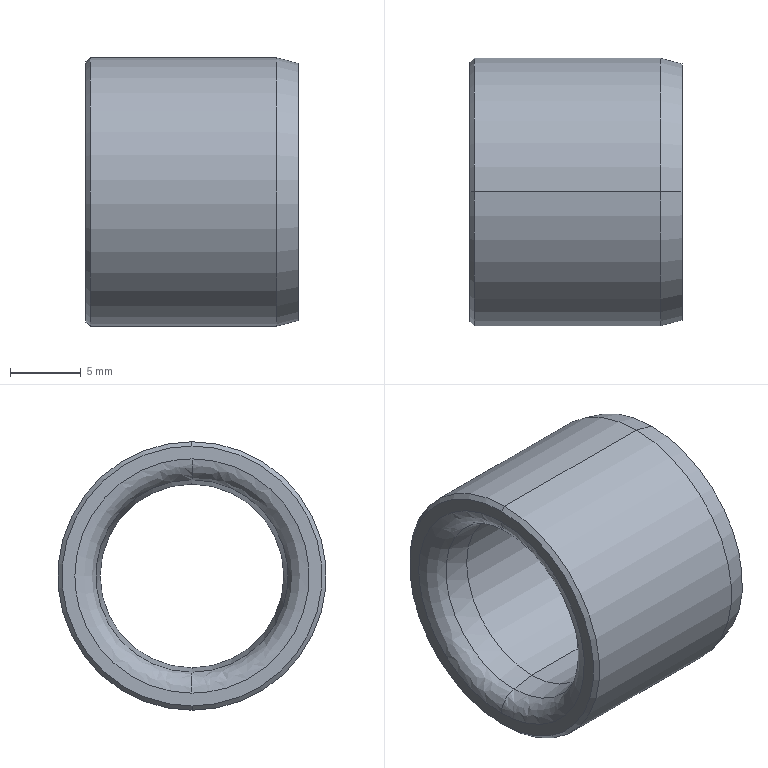Part | STEP file | TQ-DD-1105WWmpbz13_15_2_031010 | 1 solid | 18 faces | box 15 x 19 x 19 mm | volume 2146 mm3 | cone 8 | spline 4 | cylinder 4 | plane 2 | commonest cylinder face diameters 13 x2 19 x2
STEP:
#1=CARTESIAN_POINT('',(1.24,0.,6.81));
#2=VERTEX_POINT('',#1);
#3=CARTESIAN_POINT('',(1.24,0.,-6.81));
#4=VERTEX_POINT('',#3);
#5=CARTESIAN_POINT('',(1.24,0.,0.));
#6=DIRECTION('',(1.,0.,0.));
#7=DIRECTION('',(0.,0.,1.));
#8=AXIS2_PLACEMENT_3D('',#5,#6,#7);
#9=CIRCLE('',#8,6.81);
#10=EDGE_CURVE('',#2,#4,#9,.T.);
#11=ORIENTED_EDGE('',*,*,#10,.T.);
#12=CARTESIAN_POINT('',(0.,0.,-8.288));
#13=VERTEX_POINT('',#12);
#14=CARTESIAN_POINT('',(1.5,0.,-8.288));
#15=DIRECTION('',(0.,-1.,0.));
#16=DIRECTION('',(0.,0.,-1.));
#17=AXIS2_PLACEMENT_3D('',#14,#15,#16);
#18=CIRCLE('',#17,1.5);
#19=EDGE_CURVE('',#4,#13,#18,.T.);
#20=ORIENTED_EDGE('',*,*,#19,.T.);
#21=CARTESIAN_POINT('',(0.,0.,8.288));
#22=VERTEX_POINT('',#21);
#23=CARTESIAN_POINT('',(0.,0.,8.288));
#24=CARTESIAN_POINT('',(0.,-0.2535,8.288));
#25=CARTESIAN_POINT('',(0.,-0.6322,8.27));
#26=CARTESIAN_POINT('',(0.,-1.071,8.22));
#27=CARTESIAN_POINT('',(0.,-1.29,8.187));
#28=CARTESIAN_POINT('',(0.,-1.383,8.171));
#29=CARTESIAN_POINT('',(0.,-1.446,8.161));
#30=CARTESIAN_POINT('',(0.,-1.475,8.155));
#31=CARTESIAN_POINT('',(0.,-1.772,8.1));
#32=CARTESIAN_POINT('',(0.,-2.163,8.008));
#33=CARTESIAN_POINT('',(0.,-2.61,7.868));
#34=CARTESIAN_POINT('',(0.,-2.831,7.79));
#35=CARTESIAN_POINT('',(0.,-2.925,7.754));
#36=CARTESIAN_POINT('',(0.,-2.988,7.73));
#37=CARTESIAN_POINT('',(0.,-3.018,7.719));
#38=CARTESIAN_POINT('',(0.,-3.311,7.603));
#39=CARTESIAN_POINT('',(0.,-3.692,7.429));
#40=CARTESIAN_POINT('',(0.,-4.119,7.194));
#41=CARTESIAN_POINT('',(0.,-4.298,7.086));
#42=CARTESIAN_POINT('',(0.,-4.417,7.013));
#43=CARTESIAN_POINT('',(0.,-4.475,6.976));
#44=CARTESIAN_POINT('',(0.,-5.014,6.624));
#45=CARTESIAN_POINT('',(0.,-5.456,6.265));
#46=CARTESIAN_POINT('',(0.,-6.062,5.658));
#47=CARTESIAN_POINT('',(0.,-6.349,5.341));
#48=CARTESIAN_POINT('',(0.,-6.653,4.946));
#49=CARTESIAN_POINT('',(0.,-6.776,4.772));
#50=CARTESIAN_POINT('',(0.,-6.858,4.654));
#51=CARTESIAN_POINT('',(0.,-6.898,4.594));
#52=CARTESIAN_POINT('',(0.,-7.09,4.301));
#53=CARTESIAN_POINT('',(0.,-7.301,3.94));
#54=CARTESIAN_POINT('',(0.,-7.514,3.501));
#55=CARTESIAN_POINT('',(0.,-7.613,3.277));
#56=CARTESIAN_POINT('',(0.,-7.653,3.18));
#57=CARTESIAN_POINT('',(0.,-7.68,3.116));
#58=CARTESIAN_POINT('',(0.,-7.693,3.082));
#59=CARTESIAN_POINT('',(0.,-7.805,2.801));
#60=CARTESIAN_POINT('',(0.,-7.934,2.421));
#61=CARTESIAN_POINT('',(0.,-8.053,1.968));
#62=CARTESIAN_POINT('',(0.,-8.104,1.739));
#63=CARTESIAN_POINT('',(0.,-8.124,1.64));
#64=CARTESIAN_POINT('',(0.,-8.137,1.574));
#65=CARTESIAN_POINT('',(0.,-8.144,1.539));
#66=CARTESIAN_POINT('',(0.,-8.241,1.01));
#67=CARTESIAN_POINT('',(0.,-8.288,0.5066));
#68=CARTESIAN_POINT('',(0.,-8.288,-0.2533));
#69=CARTESIAN_POINT('',(0.,-8.27,-0.6317));
#70=CARTESIAN_POINT('',(0.,-8.22,-1.071));
#71=CARTESIAN_POINT('',(0.,-8.187,-1.29));
#72=CARTESIAN_POINT('',(0.,-8.171,-1.383));
#73=CARTESIAN_POINT('',(0.,-8.161,-1.446));
#74=CARTESIAN_POINT('',(0.,-8.155,-1.475));
#75=CARTESIAN_POINT('',(0.,-8.1,-1.772));
#76=CARTESIAN_POINT('',(0.,-8.008,-2.163));
#77=CARTESIAN_POINT('',(0.,-7.868,-2.61));
#78=CARTESIAN_POINT('',(0.,-7.79,-2.831));
#79=CARTESIAN_POINT('',(0.,-7.754,-2.925));
#80=CARTESIAN_POINT('',(0.,-7.73,-2.988));
#81=CARTESIAN_POINT('',(0.,-7.719,-3.018));
#82=CARTESIAN_POINT('',(0.,-7.603,-3.311));
#83=CARTESIAN_POINT('',(0.,-7.429,-3.692));
#84=CARTESIAN_POINT('',(0.,-7.194,-4.119));
#85=CARTESIAN_POINT('',(0.,-7.086,-4.298));
#86=CARTESIAN_POINT('',(0.,-7.013,-4.417));
#87=CARTESIAN_POINT('',(0.,-6.976,-4.475));
#88=CARTESIAN_POINT('',(0.,-6.624,-5.014));
#89=CARTESIAN_POINT('',(0.,-6.265,-5.456));
#90=CARTESIAN_POINT('',(0.,-5.658,-6.062));
#91=CARTESIAN_POINT('',(0.,-5.341,-6.349));
#92=CARTESIAN_POINT('',(0.,-4.946,-6.653));
#93=CARTESIAN_POINT('',(0.,-4.772,-6.776));
#94=CARTESIAN_POINT('',(0.,-4.654,-6.858));
#95=CARTESIAN_POINT('',(0.,-4.594,-6.898));
#96=CARTESIAN_POINT('',(0.,-4.301,-7.09));
#97=CARTESIAN_POINT('',(0.,-3.94,-7.301));
#98=CARTESIAN_POINT('',(0.,-3.501,-7.514));
#99=CARTESIAN_POINT('',(0.,-3.277,-7.613));
#100=CARTESIAN_POINT('',(0.,-3.18,-7.653));
#101=CARTESIAN_POINT('',(0.,-3.116,-7.68));
#102=CARTESIAN_POINT('',(0.,-3.082,-7.693));
#103=CARTESIAN_POINT('',(0.,-2.801,-7.805));
#104=CARTESIAN_POINT('',(0.,-2.421,-7.934));
#105=CARTESIAN_POINT('',(0.,-1.968,-8.053));
#106=CARTESIAN_POINT('',(0.,-1.739,-8.104));
#107=CARTESIAN_POINT('',(0.,-1.64,-8.124));
#108=CARTESIAN_POINT('',(0.,-1.574,-8.137));
#109=CARTESIAN_POINT('',(0.,-1.539,-8.144));
#110=CARTESIAN_POINT('',(0.,-1.01,-8.241));
#111=CARTESIAN_POINT('',(0.,-0.5074,-8.288));
#112=CARTESIAN_POINT('',(0.,0.,-8.288));
#113=B_SPLINE_CURVE_WITH_KNOTS('',3,(#23,#24,#25,#26,#27,#28,#29,#30,#31,#32,#33,#34,#35,#36,#37,#38,#39,#40,#41,#42,#43,#44,#45,#46,#47,#48,#49,#50,#51,#52,#53,#54,#55,#56,#57,#58,#59,#60,#61,#62,#63,#64,#65,#66,#67,#68,#69,#70,#71,#72,#73,#74,#75,#76,#77,#78,#79,#80,#81,#82,#83,#84,#85,#86,#87,#88,#89,#90,#91,#92,#93,#94,#95,#96,#97,#98,#99,#100,#101,#102,#103,#104,#105,#106,#107,#108,#109,#110,#111,#112),.UNSPECIFIED.,.F.,.F.,(4,1,1,1,2,2,1,1,1,2,2,1,1,2,2,2,1,1,2,2,1,1,1,2,2,1,1,1,2,2,2,1,1,1,2,2,1,1,1,2,2,1,1,2,2,2,1,1,2,2,1,1,1,2,2,1,1,1,2,2,4),(0.,0.03125,0.04688,0.05469,0.05859,0.0625,0.09375,0.1094,0.1172,0.1211,0.125,0.1563,0.1719,0.1797,0.1875,0.25,0.2813,0.2969,0.3047,0.3125,0.3438,0.3594,0.3672,0.3711,0.375,0.4063,0.4219,0.4297,0.4336,0.4375,0.5,0.5313,0.5469,0.5547,0.5586,0.5625,0.5938,0.6094,0.6172,0.6211,0.625,0.6563,0.6719,0.6797,0.6875,0.75,0.7813,0.7969,0.8047,0.8125,0.8437,0.8594,0.8672,0.8711,0.875,0.9063,0.9219,0.9297,0.9336,0.9375,1.),.UNSPECIFIED.);
#114=EDGE_CURVE('',#22,#13,#113,.T.);
#115=ORIENTED_EDGE('',*,*,#114,.F.);
#116=CARTESIAN_POINT('',(1.5,0.,8.288));
#117=DIRECTION('',(0.,1.,0.));
#118=DIRECTION('',(0.,0.,1.));
#119=AXIS2_PLACEMENT_3D('',#116,#117,#118);
#120=CIRCLE('',#119,1.5);
#121=EDGE_CURVE('',#2,#22,#120,.T.);
#122=ORIENTED_EDGE('',*,*,#121,.F.);
#123=EDGE_LOOP('',(#11,#20,#115,#122));
#124=FACE_OUTER_BOUND('',#123,.T.);
#125=CARTESIAN_POINT('',(1.24,0.,-6.81));
#126=CARTESIAN_POINT('',(1.24,-13.621,-6.81));
#127=CARTESIAN_POINT('',(1.24,-13.621,6.81));
#128=CARTESIAN_POINT('',(1.24,0.,6.81));
#129=CARTESIAN_POINT('',(0.4895,0.,-6.943));
#130=CARTESIAN_POINT('',(0.4895,-13.885,-6.943));
#131=CARTESIAN_POINT('',(0.4895,-13.885,6.943));
#132=CARTESIAN_POINT('',(0.4895,0.,6.943));
#133=CARTESIAN_POINT('',(0.,0.,-7.526));
#134=CARTESIAN_POINT('',(0.,-15.052,-7.526));
#135=CARTESIAN_POINT('',(0.,-15.052,7.526));
#136=CARTESIAN_POINT('',(0.,0.,7.526));
#137=CARTESIAN_POINT('',(0.,0.,-8.288));
#138=CARTESIAN_POINT('',(0.,-16.575,-8.288));
#139=CARTESIAN_POINT('',(0.,-16.575,8.288));
#140=CARTESIAN_POINT('',(0.,0.,8.288));
#141=(BOUNDED_SURFACE()B_SPLINE_SURFACE(3,3,((#125,#126,#127,#128),(#129,#130,#131,#132),(#133,#134,#135,#136),(#137,#138,#139,#140)),.UNSPECIFIED.,.F.,.F.,.F.)B_SPLINE_SURFACE_WITH_KNOTS((4,4),(4,4),(0.,1.),(0.,1.),.UNSPECIFIED.)GEOMETRIC_REPRESENTATION_ITEM()RATIONAL_B_SPLINE_SURFACE(((1.,0.3333,0.3333,1.),(0.844,0.2813,0.2813,0.844),(0.844,0.2813,0.2813,0.844),(1.,0.3333,0.3333,1.)))REPRESENTATION_ITEM('')SURFACE());
#142=ADVANCED_FACE('',(#124),#141,.T.);
#143=CARTESIAN_POINT('',(15.,0.,-8.288));
#144=VERTEX_POINT('',#143);
#145=CARTESIAN_POINT('',(15.,0.,8.288));
#146=VERTEX_POINT('',#145);
#147=CARTESIAN_POINT('',(15.,0.,-8.288));
#148=CARTESIAN_POINT('',(15.,-0.2535,-8.288));
#149=CARTESIAN_POINT('',(15.,-0.6322,-8.27));
#150=CARTESIAN_POINT('',(15.,-1.071,-8.22));
#151=CARTESIAN_POINT('',(15.,-1.29,-8.187));
#152=CARTESIAN_POINT('',(15.,-1.383,-8.171));
#153=CARTESIAN_POINT('',(15.,-1.446,-8.161));
#154=CARTESIAN_POINT('',(15.,-1.475,-8.155));
#155=CARTESIAN_POINT('',(15.,-1.772,-8.1));
#156=CARTESIAN_POINT('',(15.,-2.163,-8.008));
#157=CARTESIAN_POINT('',(15.,-2.61,-7.868));
#158=CARTESIAN_POINT('',(15.,-2.831,-7.79));
#159=CARTESIAN_POINT('',(15.,-2.925,-7.754));
#160=CARTESIAN_POINT('',(15.,-2.988,-7.73));
#161=CARTESIAN_POINT('',(15.,-3.018,-7.719));
#162=CARTESIAN_POINT('',(15.,-3.311,-7.603));
#163=CARTESIAN_POINT('',(15.,-3.692,-7.429));
#164=CARTESIAN_POINT('',(15.,-4.119,-7.194));
#165=CARTESIAN_POINT('',(15.,-4.298,-7.086));
#166=CARTESIAN_POINT('',(15.,-4.417,-7.013));
#167=CARTESIAN_POINT('',(15.,-4.475,-6.976));
#168=CARTESIAN_POINT('',(15.,-5.014,-6.624));
#169=CARTESIAN_POINT('',(15.,-5.456,-6.265));
#170=CARTESIAN_POINT('',(15.,-6.062,-5.658));
#171=CARTESIAN_POINT('',(15.,-6.349,-5.341));
#172=CARTESIAN_POINT('',(15.,-6.653,-4.946));
#173=CARTESIAN_POINT('',(15.,-6.776,-4.772));
#174=CARTESIAN_POINT('',(15.,-6.858,-4.654));
#175=CARTESIAN_POINT('',(15.,-6.898,-4.594));
#176=CARTESIAN_POINT('',(15.,-7.09,-4.301));
#177=CARTESIAN_POINT('',(15.,-7.301,-3.94));
#178=CARTESIAN_POINT('',(15.,-7.514,-3.501));
#179=CARTESIAN_POINT('',(15.,-7.613,-3.277));
#180=CARTESIAN_POINT('',(15.,-7.653,-3.18));
#181=CARTESIAN_POINT('',(15.,-7.68,-3.116));
#182=CARTESIAN_POINT('',(15.,-7.693,-3.082));
#183=CARTESIAN_POINT('',(15.,-7.805,-2.801));
#184=CARTESIAN_POINT('',(15.,-7.934,-2.421));
#185=CARTESIAN_POINT('',(15.,-8.053,-1.968));
#186=CARTESIAN_POINT('',(15.,-8.104,-1.739));
#187=CARTESIAN_POINT('',(15.,-8.124,-1.64));
#188=CARTESIAN_POINT('',(15.,-8.137,-1.574));
#189=CARTESIAN_POINT('',(15.,-8.144,-1.539));
#190=CARTESIAN_POINT('',(15.,-8.241,-1.01));
#191=CARTESIAN_POINT('',(15.,-8.288,-0.5066));
#192=CARTESIAN_POINT('',(15.,-8.288,0.2533));
#193=CARTESIAN_POINT('',(15.,-8.27,0.6317));
#194=CARTESIAN_POINT('',(15.,-8.22,1.071));
#195=CARTESIAN_POINT('',(15.,-8.187,1.29));
#196=CARTESIAN_POINT('',(15.,-8.171,1.383));
#197=CARTESIAN_POINT('',(15.,-8.161,1.446));
#198=CARTESIAN_POINT('',(15.,-8.155,1.475));
#199=CARTESIAN_POINT('',(15.,-8.1,1.772));
#200=CARTESIAN_POINT('',(15.,-8.008,2.163));
#201=CARTESIAN_POINT('',(15.,-7.868,2.61));
#202=CARTESIAN_POINT('',(15.,-7.79,2.831));
#203=CARTESIAN_POINT('',(15.,-7.754,2.925));
#204=CARTESIAN_POINT('',(15.,-7.73,2.988));
#205=CARTESIAN_POINT('',(15.,-7.719,3.018));
#206=CARTESIAN_POINT('',(15.,-7.603,3.311));
#207=CARTESIAN_POINT('',(15.,-7.429,3.692));
#208=CARTESIAN_POINT('',(15.,-7.194,4.119));
#209=CARTESIAN_POINT('',(15.,-7.086,4.298));
#210=CARTESIAN_POINT('',(15.,-7.013,4.417));
#211=CARTESIAN_POINT('',(15.,-6.976,4.475));
#212=CARTESIAN_POINT('',(15.,-6.624,5.014));
#213=CARTESIAN_POINT('',(15.,-6.265,5.456));
#214=CARTESIAN_POINT('',(15.,-5.658,6.062));
#215=CARTESIAN_POINT('',(15.,-5.341,6.349));
#216=CARTESIAN_POINT('',(15.,-4.946,6.653));
#217=CARTESIAN_POINT('',(15.,-4.772,6.776));
#218=CARTESIAN_POINT('',(15.,-4.654,6.858));
#219=CARTESIAN_POINT('',(15.,-4.594,6.898));
#220=CARTESIAN_POINT('',(15.,-4.301,7.09));
#221=CARTESIAN_POINT('',(15.,-3.94,7.301));
#222=CARTESIAN_POINT('',(15.,-3.501,7.514));
#223=CARTESIAN_POINT('',(15.,-3.277,7.613));
#224=CARTESIAN_POINT('',(15.,-3.18,7.653));
#225=CARTESIAN_POINT('',(15.,-3.116,7.68));
#226=CARTESIAN_POINT('',(15.,-3.082,7.693));
#227=CARTESIAN_POINT('',(15.,-2.801,7.805));
#228=CARTESIAN_POINT('',(15.,-2.421,7.934));
#229=CARTESIAN_POINT('',(15.,-1.968,8.053));
#230=CARTESIAN_POINT('',(15.,-1.739,8.104));
#231=CARTESIAN_POINT('',(15.,-1.64,8.124));
#232=CARTESIAN_POINT('',(15.,-1.574,8.137));
#233=CARTESIAN_POINT('',(15.,-1.539,8.144));
#234=CARTESIAN_POINT('',(15.,-1.01,8.241));
#235=CARTESIAN_POINT('',(15.,-0.5074,8.288));
#236=CARTESIAN_POINT('',(15.,0.,8.288));
#237=B_SPLINE_CURVE_WITH_KNOTS('',3,(#147,#148,#149,#150,#151,#152,#153,#154,#155,#156,#157,#158,#159,#160,#161,#162,#163,#164,#165,#166,#167,#168,#169,#170,#171,#172,#173,#174,#175,#176,#177,#178,#179,#180,#181,#182,#183,#184,#185,#186,#187,#188,#189,#190,#191,#192,#193,#194,#195,#196,#197,#198,#199,#200,#201,#202,#203,#204,#205,#206,#207,#208,#209,#210,#211,#212,#213,#214,#215,#216,#217,#218,#219,#220,#221,#222,#223,#224,#225,#226,#227,#228,#229,#230,#231,#232,#233,#234,#235,#236),.UNSPECIFIED.,.F.,.F.,(4,1,1,1,2,2,1,1,1,2,2,1,1,2,2,2,1,1,2,2,1,1,1,2,2,1,1,1,2,2,2,1,1,1,2,2,1,1,1,2,2,1,1,2,2,2,1,1,2,2,1,1,1,2,2,1,1,1,2,2,4),(0.,0.03125,0.04687,0.05469,0.05859,0.0625,0.09375,0.1094,0.1172,0.1211,0.125,0.1563,0.1719,0.1797,0.1875,0.25,0.2813,0.2969,0.3047,0.3125,0.3437,0.3594,0.3672,0.3711,0.375,0.4062,0.4219,0.4297,0.4336,0.4375,0.5,0.5312,0.5469,0.5547,0.5586,0.5625,0.5937,0.6094,0.6172,0.6211,0.625,0.6562,0.6719,0.6797,0.6875,0.75,0.7812,0.7969,0.8047,0.8125,0.8438,0.8594,0.8672,0.8711,0.875,0.9063,0.9219,0.9297,0.9336,0.9375,1.),.UNSPECIFIED.);
#238=EDGE_CURVE('',#144,#146,#237,.T.);
#239=ORIENTED_EDGE('',*,*,#238,.F.);
#240=CARTESIAN_POINT('',(13.76,0.,-6.81));
#241=VERTEX_POINT('',#240);
#242=CARTESIAN_POINT('',(13.5,0.,-8.288));
#243=DIRECTION('',(0.,-1.,0.));
#244=DIRECTION('',(0.,0.,-1.));
#245=AXIS2_PLACEMENT_3D('',#242,#243,#244);
#246=CIRCLE('',#245,1.5);
#247=EDGE_CURVE('',#144,#241,#246,.T.);
#248=ORIENTED_EDGE('',*,*,#247,.T.);
#249=CARTESIAN_POINT('',(13.76,0.,6.81));
#250=VERTEX_POINT('',#249);
#251=CARTESIAN_POINT('',(13.76,0.,0.));
#252=DIRECTION('',(-1.,0.,0.));
#253=DIRECTION('',(0.,0.,1.));
#254=AXIS2_PLACEMENT_3D('',#251,#252,#253);
#255=CIRCLE('',#254,6.81);
#256=EDGE_CURVE('',#241,#250,#255,.T.);
#257=ORIENTED_EDGE('',*,*,#256,.T.);
#258=CARTESIAN_POINT('',(13.5,0.,8.288));
#259=DIRECTION('',(0.,1.,0.));
#260=DIRECTION('',(0.,0.,1.));
#261=AXIS2_PLACEMENT_3D('',#258,#259,#260);
#262=CIRCLE('',#261,1.5);
#263=EDGE_CURVE('',#146,#250,#262,.T.);
#264=ORIENTED_EDGE('',*,*,#263,.F.);
#265=EDGE_LOOP('',(#239,#248,#257,#264));
#266=FACE_OUTER_BOUND('',#265,.T.);
#267=CARTESIAN_POINT('',(15.,0.,-8.288));
#268=CARTESIAN_POINT('',(15.,-16.575,-8.288));
#269=CARTESIAN_POINT('',(15.,-16.575,8.288));
#270=CARTESIAN_POINT('',(15.,0.,8.288));
#271=CARTESIAN_POINT('',(15.,0.,-7.526));
#272=CARTESIAN_POINT('',(15.,-15.052,-7.526));
#273=CARTESIAN_POINT('',(15.,-15.052,7.526));
#274=CARTESIAN_POINT('',(15.,0.,7.526));
#275=CARTESIAN_POINT('',(14.51,0.,-6.943));
#276=CARTESIAN_POINT('',(14.51,-13.885,-6.943));
#277=CARTESIAN_POINT('',(14.51,-13.885,6.943));
#278=CARTESIAN_POINT('',(14.51,0.,6.943));
#279=CARTESIAN_POINT('',(13.76,0.,-6.81));
#280=CARTESIAN_POINT('',(13.76,-13.621,-6.81));
#281=CARTESIAN_POINT('',(13.76,-13.621,6.81));
#282=CARTESIAN_POINT('',(13.76,0.,6.81));
#283=(BOUNDED_SURFACE()B_SPLINE_SURFACE(3,3,((#267,#268,#269,#270),(#271,#272,#273,#274),(#275,#276,#277,#278),(#279,#280,#281,#282)),.UNSPECIFIED.,.F.,.F.,.F.)B_SPLINE_SURFACE_WITH_KNOTS((4,4),(4,4),(0.,1.),(0.,1.),.UNSPECIFIED.)GEOMETRIC_REPRESENTATION_ITEM()RATIONAL_B_SPLINE_SURFACE(((1.,0.3333,0.3333,1.),(0.844,0.2813,0.2813,0.844),(0.844,0.2813,0.2813,0.844),(1.,0.3333,0.3333,1.)))REPRESENTATION_ITEM('')SURFACE());
#284=ADVANCED_FACE('',(#266),#283,.T.);
#285=CARTESIAN_POINT('',(0.3,0.,-9.5));
#286=VERTEX_POINT('',#285);
#287=CARTESIAN_POINT('',(0.3,0.,9.5));
#288=VERTEX_POINT('',#287);
#289=CARTESIAN_POINT('',(0.3,0.,0.));
#290=DIRECTION('',(1.,0.,0.));
#291=DIRECTION('',(0.,0.,-1.));
#292=AXIS2_PLACEMENT_3D('',#289,#290,#291);
#293=CIRCLE('',#292,9.5);
#294=EDGE_CURVE('',#286,#288,#293,.T.);
#295=ORIENTED_EDGE('',*,*,#294,.T.);
#296=CARTESIAN_POINT('',(13.5,0.,9.5));
#297=VERTEX_POINT('',#296);
#298=CARTESIAN_POINT('',(6.9,0.,9.5));
#299=DIRECTION('',(1.,0.,0.));
#300=VECTOR('',#299,1000.);
#301=LINE('',#298,#300);
#302=EDGE_CURVE('',#288,#297,#301,.T.);
#303=ORIENTED_EDGE('',*,*,#302,.T.);
#304=CARTESIAN_POINT('',(13.5,0.,-9.5));
#305=VERTEX_POINT('',#304);
#306=CARTESIAN_POINT('',(13.5,0.,0.));
#307=DIRECTION('',(-1.,0.,0.));
#308=DIRECTION('',(0.,0.,-1.));
#309=AXIS2_PLACEMENT_3D('',#306,#307,#308);
#310=CIRCLE('',#309,9.5);
#311=EDGE_CURVE('',#297,#305,#310,.T.);
#312=ORIENTED_EDGE('',*,*,#311,.T.);
#313=CARTESIAN_POINT('',(6.9,0.,-9.5));
#314=DIRECTION('',(1.,0.,0.));
#315=VECTOR('',#314,1000.);
#316=LINE('',#313,#315);
#317=EDGE_CURVE('',#286,#305,#316,.T.);
#318=ORIENTED_EDGE('',*,*,#317,.F.);
#319=EDGE_LOOP('',(#295,#303,#312,#318));
#320=FACE_OUTER_BOUND('',#319,.T.);
#321=CARTESIAN_POINT('',(6.9,0.,0.));
#322=DIRECTION('',(1.,0.,0.));
#323=DIRECTION('',(0.,0.,-1.));
#324=AXIS2_PLACEMENT_3D('',#321,#322,#323);
#325=CYLINDRICAL_SURFACE('',#324,9.5);
#326=ADVANCED_FACE('',(#320),#325,.T.);
#327=CARTESIAN_POINT('',(0.,0.,-9.2));
#328=VERTEX_POINT('',#327);
#329=CARTESIAN_POINT('',(0.,0.,9.2));
#330=VERTEX_POINT('',#329);
#331=CARTESIAN_POINT('',(0.,0.,0.));
#332=DIRECTION('',(1.,0.,0.));
#333=DIRECTION('',(0.,0.,-1.));
#334=AXIS2_PLACEMENT_3D('',#331,#332,#333);
#335=CIRCLE('',#334,9.2);
#336=EDGE_CURVE('',#328,#330,#335,.T.);
#337=ORIENTED_EDGE('',*,*,#336,.T.);
#338=CARTESIAN_POINT('',(0.3,0.,9.5));
#339=DIRECTION('',(0.7071,0.,0.7071));
#340=VECTOR('',#339,1000.);
#341=LINE('',#338,#340);
#342=EDGE_CURVE('',#330,#288,#341,.T.);
#343=ORIENTED_EDGE('',*,*,#342,.T.);
#344=ORIENTED_EDGE('',*,*,#294,.F.);
#345=CARTESIAN_POINT('',(0.3,0.,-9.5));
#346=DIRECTION('',(0.7071,0.,-0.7071));
#347=VECTOR('',#346,1000.);
#348=LINE('',#345,#347);
#349=EDGE_CURVE('',#328,#286,#348,.T.);
#350=ORIENTED_EDGE('',*,*,#349,.F.);
#351=EDGE_LOOP('',(#337,#343,#344,#350));
#352=FACE_OUTER_BOUND('',#351,.T.);
#353=CARTESIAN_POINT('',(0.3,0.,0.));
#354=DIRECTION('',(1.,0.,0.));
#355=DIRECTION('',(0.,0.,-1.));
#356=AXIS2_PLACEMENT_3D('',#353,#354,#355);
#357=CONICAL_SURFACE('',#356,9.5,0.7854);
#358=ADVANCED_FACE('',(#352),#357,.T.);
#359=CARTESIAN_POINT('',(15.,0.,9.098));
#360=VERTEX_POINT('',#359);
#361=CARTESIAN_POINT('',(15.,0.,-9.098));
#362=VERTEX_POINT('',#361);
#363=CARTESIAN_POINT('',(15.,0.,0.));
#364=DIRECTION('',(-1.,0.,0.));
#365=DIRECTION('',(0.,0.,1.));
#366=AXIS2_PLACEMENT_3D('',#363,#364,#365);
#367=CIRCLE('',#366,9.098);
#368=EDGE_CURVE('',#360,#362,#367,.T.);
#369=ORIENTED_EDGE('',*,*,#368,.T.);
#370=CARTESIAN_POINT('',(13.5,0.,-9.5));
#371=DIRECTION('',(-0.9659,0.,-0.2588));
#372=VECTOR('',#371,1000.);
#373=LINE('',#370,#372);
#374=EDGE_CURVE('',#362,#305,#373,.T.);
#375=ORIENTED_EDGE('',*,*,#374,.T.);
#376=ORIENTED_EDGE('',*,*,#311,.F.);
#377=CARTESIAN_POINT('',(13.5,0.,9.5));
#378=DIRECTION('',(-0.9659,0.,0.2588));
#379=VECTOR('',#378,1000.);
#380=LINE('',#377,#379);
#381=EDGE_CURVE('',#360,#297,#380,.T.);
#382=ORIENTED_EDGE('',*,*,#381,.F.);
#383=EDGE_LOOP('',(#369,#375,#376,#382));
#384=FACE_OUTER_BOUND('',#383,.T.);
#385=CARTESIAN_POINT('',(13.5,0.,0.));
#386=DIRECTION('',(-1.,0.,0.));
#387=DIRECTION('',(0.,0.,1.));
#388=AXIS2_PLACEMENT_3D('',#385,#386,#387);
#389=CONICAL_SURFACE('',#388,9.5,0.2618);
#390=ADVANCED_FACE('',(#384),#389,.T.);
#391=CARTESIAN_POINT('',(3.,0.,-6.5));
#392=VERTEX_POINT('',#391);
#393=CARTESIAN_POINT('',(3.,0.,6.5));
#394=VERTEX_POINT('',#393);
#395=CARTESIAN_POINT('',(3.,0.,0.));
#396=DIRECTION('',(-1.,0.,0.));
#397=DIRECTION('',(0.,1.,0.));
#398=AXIS2_PLACEMENT_3D('',#395,#396,#397);
#399=CIRCLE('',#398,6.5);
#400=EDGE_CURVE('',#392,#394,#399,.T.);
#401=ORIENTED_EDGE('',*,*,#400,.F.);
#402=CARTESIAN_POINT('',(1.24,0.,-6.81));
#403=DIRECTION('',(-0.9848,0.,-0.1736));
#404=VECTOR('',#403,1000.);
#405=LINE('',#402,#404);
#406=EDGE_CURVE('',#392,#4,#405,.T.);
#407=ORIENTED_EDGE('',*,*,#406,.T.);
#408=ORIENTED_EDGE('',*,*,#10,.F.);
#409=CARTESIAN_POINT('',(1.24,0.,6.81));
#410=DIRECTION('',(-0.9848,0.,0.1736));
#411=VECTOR('',#410,1000.);
#412=LINE('',#409,#411);
#413=EDGE_CURVE('',#394,#2,#412,.T.);
#414=ORIENTED_EDGE('',*,*,#413,.F.);
#415=EDGE_LOOP('',(#401,#407,#408,#414));
#416=FACE_OUTER_BOUND('',#415,.T.);
#417=CARTESIAN_POINT('',(1.24,0.,0.));
#418=DIRECTION('',(-1.,0.,0.));
#419=DIRECTION('',(0.,0.,1.));
#420=AXIS2_PLACEMENT_3D('',#417,#418,#419);
#421=CONICAL_SURFACE('',#420,6.81,0.1745);
#422=ADVANCED_FACE('',(#416),#421,.F.);
#423=CARTESIAN_POINT('',(12.,0.,6.5));
#424=VERTEX_POINT('',#423);
#425=CARTESIAN_POINT('',(12.,0.,-6.5));
#426=VERTEX_POINT('',#425);
#427=CARTESIAN_POINT('',(12.,0.,0.));
#428=DIRECTION('',(1.,0.,0.));
#429=DIRECTION('',(0.,1.,0.));
#430=AXIS2_PLACEMENT_3D('',#427,#428,#429);
#431=CIRCLE('',#430,6.5);
#432=EDGE_CURVE('',#424,#426,#431,.T.);
#433=ORIENTED_EDGE('',*,*,#432,.F.);
#434=CARTESIAN_POINT('',(13.76,0.,6.81));
#435=DIRECTION('',(0.9848,0.,0.1736));
#436=VECTOR('',#435,1000.);
#437=LINE('',#434,#436);
#438=EDGE_CURVE('',#424,#250,#437,.T.);
#439=ORIENTED_EDGE('',*,*,#438,.T.);
#440=ORIENTED_EDGE('',*,*,#256,.F.);
#441=CARTESIAN_POINT('',(13.76,0.,-6.81));
#442=DIRECTION('',(0.9848,0.,-0.1736));
#443=VECTOR('',#442,1000.);
#444=LINE('',#441,#443);
#445=EDGE_CURVE('',#426,#241,#444,.T.);
#446=ORIENTED_EDGE('',*,*,#445,.F.);
#447=EDGE_LOOP('',(#433,#439,#440,#446));
#448=FACE_OUTER_BOUND('',#447,.T.);
#449=CARTESIAN_POINT('',(13.76,0.,0.));
#450=DIRECTION('',(1.,0.,0.));
#451=DIRECTION('',(0.,0.,-1.));
#452=AXIS2_PLACEMENT_3D('',#449,#450,#451);
#453=CONICAL_SURFACE('',#452,6.81,0.1745);
#454=ADVANCED_FACE('',(#448),#453,.F.);
#455=ORIENTED_EDGE('',*,*,#400,.T.);
#456=CARTESIAN_POINT('',(7.5,0.,6.5));
#457=DIRECTION('',(1.,0.,0.));
#458=VECTOR('',#457,1000.);
#459=LINE('',#456,#458);
#460=EDGE_CURVE('',#394,#424,#459,.T.);
#461=ORIENTED_EDGE('',*,*,#460,.T.);
#462=ORIENTED_EDGE('',*,*,#432,.T.);
#463=CARTESIAN_POINT('',(7.5,0.,-6.5));
#464=DIRECTION('',(1.,0.,0.));
#465=VECTOR('',#464,1000.);
#466=LINE('',#463,#465);
#467=EDGE_CURVE('',#392,#426,#466,.T.);
#468=ORIENTED_EDGE('',*,*,#467,.F.);
#469=EDGE_LOOP('',(#455,#461,#462,#468));
#470=FACE_OUTER_BOUND('',#469,.T.);
#471=CARTESIAN_POINT('',(7.5,0.,0.));
#472=DIRECTION('',(1.,0.,0.));
#473=DIRECTION('',(0.,0.,-1.));
#474=AXIS2_PLACEMENT_3D('',#471,#472,#473);
#475=CYLINDRICAL_SURFACE('',#474,6.5);
#476=ADVANCED_FACE('',(#470),#475,.F.);
#477=ORIENTED_EDGE('',*,*,#302,.F.);
#478=CARTESIAN_POINT('',(0.3,0.,0.));
#479=DIRECTION('',(1.,0.,0.));
#480=DIRECTION('',(0.,0.,-1.));
#481=AXIS2_PLACEMENT_3D('',#478,#479,#480);
#482=CIRCLE('',#481,9.5);
#483=EDGE_CURVE('',#288,#286,#482,.T.);
#484=ORIENTED_EDGE('',*,*,#483,.T.);
#485=ORIENTED_EDGE('',*,*,#317,.T.);
#486=CARTESIAN_POINT('',(13.5,0.,0.));
#487=DIRECTION('',(-1.,0.,0.));
#488=DIRECTION('',(0.,0.,-1.));
#489=AXIS2_PLACEMENT_3D('',#486,#487,#488);
#490=CIRCLE('',#489,9.5);
#491=EDGE_CURVE('',#305,#297,#490,.T.);
#492=ORIENTED_EDGE('',*,*,#491,.T.);
#493=EDGE_LOOP('',(#477,#484,#485,#492));
#494=FACE_OUTER_BOUND('',#493,.T.);
#495=CARTESIAN_POINT('',(6.9,0.,0.));
#496=DIRECTION('',(1.,0.,0.));
#497=DIRECTION('',(0.,0.,-1.));
#498=AXIS2_PLACEMENT_3D('',#495,#496,#497);
#499=CYLINDRICAL_SURFACE('',#498,9.5);
#500=ADVANCED_FACE('',(#494),#499,.T.);
#501=ORIENTED_EDGE('',*,*,#342,.F.);
#502=CARTESIAN_POINT('',(0.,0.,0.));
#503=DIRECTION('',(1.,0.,0.));
#504=DIRECTION('',(0.,0.,-1.));
#505=AXIS2_PLACEMENT_3D('',#502,#503,#504);
#506=CIRCLE('',#505,9.2);
#507=EDGE_CURVE('',#330,#328,#506,.T.);
#508=ORIENTED_EDGE('',*,*,#507,.T.);
#509=ORIENTED_EDGE('',*,*,#349,.T.);
#510=ORIENTED_EDGE('',*,*,#483,.F.);
#511=EDGE_LOOP('',(#501,#508,#509,#510));
#512=FACE_OUTER_BOUND('',#511,.T.);
#513=CARTESIAN_POINT('',(0.3,0.,0.));
#514=DIRECTION('',(1.,0.,0.));
#515=DIRECTION('',(0.,0.,-1.));
#516=AXIS2_PLACEMENT_3D('',#513,#514,#515);
#517=CONICAL_SURFACE('',#516,9.5,0.7854);
#518=ADVANCED_FACE('',(#512),#517,.T.);
#519=ORIENTED_EDGE('',*,*,#374,.F.);
#520=CARTESIAN_POINT('',(15.,0.,0.));
#521=DIRECTION('',(-1.,0.,0.));
#522=DIRECTION('',(0.,0.,1.));
#523=AXIS2_PLACEMENT_3D('',#520,#521,#522);
#524=CIRCLE('',#523,9.098);
#525=EDGE_CURVE('',#362,#360,#524,.T.);
#526=ORIENTED_EDGE('',*,*,#525,.T.);
#527=ORIENTED_EDGE('',*,*,#381,.T.);
#528=ORIENTED_EDGE('',*,*,#491,.F.);
#529=EDGE_LOOP('',(#519,#526,#527,#528));
#530=FACE_OUTER_BOUND('',#529,.T.);
#531=CARTESIAN_POINT('',(13.5,0.,0.));
#532=DIRECTION('',(-1.,0.,0.));
#533=DIRECTION('',(0.,0.,1.));
#534=AXIS2_PLACEMENT_3D('',#531,#532,#533);
#535=CONICAL_SURFACE('',#534,9.5,0.2618);
#536=ADVANCED_FACE('',(#530),#535,.T.);
#537=ORIENTED_EDGE('',*,*,#336,.F.);
#538=ORIENTED_EDGE('',*,*,#507,.F.);
#539=EDGE_LOOP('',(#537,#538));
#540=FACE_OUTER_BOUND('',#539,.T.);
#541=CARTESIAN_POINT('',(0.,8.288,0.));
#542=VERTEX_POINT('',#541);
#543=CARTESIAN_POINT('',(0.,8.288,0.));
#544=CARTESIAN_POINT('',(0.,8.288,0.2535));
#545=CARTESIAN_POINT('',(0.,8.27,0.6322));
#546=CARTESIAN_POINT('',(0.,8.22,1.071));
#547=CARTESIAN_POINT('',(0.,8.187,1.29));
#548=CARTESIAN_POINT('',(0.,8.171,1.383));
#549=CARTESIAN_POINT('',(0.,8.161,1.446));
#550=CARTESIAN_POINT('',(0.,8.155,1.475));
#551=CARTESIAN_POINT('',(0.,8.1,1.772));
#552=CARTESIAN_POINT('',(0.,8.008,2.163));
#553=CARTESIAN_POINT('',(0.,7.868,2.61));
#554=CARTESIAN_POINT('',(0.,7.79,2.831));
#555=CARTESIAN_POINT('',(0.,7.754,2.925));
#556=CARTESIAN_POINT('',(0.,7.73,2.988));
#557=CARTESIAN_POINT('',(0.,7.719,3.018));
#558=CARTESIAN_POINT('',(0.,7.603,3.311));
#559=CARTESIAN_POINT('',(0.,7.429,3.692));
#560=CARTESIAN_POINT('',(0.,7.194,4.119));
#561=CARTESIAN_POINT('',(0.,7.086,4.298));
#562=CARTESIAN_POINT('',(0.,7.013,4.417));
#563=CARTESIAN_POINT('',(0.,6.976,4.475));
#564=CARTESIAN_POINT('',(0.,6.624,5.014));
#565=CARTESIAN_POINT('',(0.,6.265,5.456));
#566=CARTESIAN_POINT('',(0.,5.658,6.062));
#567=CARTESIAN_POINT('',(0.,5.341,6.349));
#568=CARTESIAN_POINT('',(0.,4.946,6.653));
#569=CARTESIAN_POINT('',(0.,4.772,6.776));
#570=CARTESIAN_POINT('',(0.,4.654,6.858));
#571=CARTESIAN_POINT('',(0.,4.594,6.898));
#572=CARTESIAN_POINT('',(0.,4.301,7.09));
#573=CARTESIAN_POINT('',(0.,3.94,7.301));
#574=CARTESIAN_POINT('',(0.,3.501,7.514));
#575=CARTESIAN_POINT('',(0.,3.277,7.613));
#576=CARTESIAN_POINT('',(0.,3.18,7.653));
#577=CARTESIAN_POINT('',(0.,3.116,7.68));
#578=CARTESIAN_POINT('',(0.,3.082,7.693));
#579=CARTESIAN_POINT('',(0.,2.801,7.805));
#580=CARTESIAN_POINT('',(0.,2.421,7.934));
#581=CARTESIAN_POINT('',(0.,1.968,8.053));
#582=CARTESIAN_POINT('',(0.,1.739,8.104));
#583=CARTESIAN_POINT('',(0.,1.64,8.124));
#584=CARTESIAN_POINT('',(0.,1.574,8.137));
#585=CARTESIAN_POINT('',(0.,1.539,8.144));
#586=CARTESIAN_POINT('',(0.,1.01,8.241));
#587=CARTESIAN_POINT('',(0.,0.5074,8.288));
#588=CARTESIAN_POINT('',(0.,0.,8.288));
#589=B_SPLINE_CURVE_WITH_KNOTS('',3,(#543,#544,#545,#546,#547,#548,#549,#550,#551,#552,#553,#554,#555,#556,#557,#558,#559,#560,#561,#562,#563,#564,#565,#566,#567,#568,#569,#570,#571,#572,#573,#574,#575,#576,#577,#578,#579,#580,#581,#582,#583,#584,#585,#586,#587,#588),.UNSPECIFIED.,.F.,.F.,(4,1,1,1,2,2,1,1,1,2,2,1,1,2,2,2,1,1,2,2,1,1,1,2,2,1,1,1,2,2,4),(0.,0.0625,0.09375,0.1094,0.1172,0.125,0.1875,0.2188,0.2344,0.2422,0.25,0.3125,0.3438,0.3594,0.375,0.5,0.5625,0.5938,0.6094,0.625,0.6875,0.7188,0.7344,0.7422,0.75,0.8125,0.8437,0.8594,0.8672,0.875,1.),.UNSPECIFIED.);
#590=EDGE_CURVE('',#542,#22,#589,.T.);
#591=ORIENTED_EDGE('',*,*,#590,.T.);
#592=ORIENTED_EDGE('',*,*,#114,.T.);
#593=CARTESIAN_POINT('',(0.,0.,-8.288));
#594=CARTESIAN_POINT('',(0.,0.2535,-8.288));
#595=CARTESIAN_POINT('',(0.,0.6322,-8.27));
#596=CARTESIAN_POINT('',(0.,1.071,-8.22));
#597=CARTESIAN_POINT('',(0.,1.29,-8.187));
#598=CARTESIAN_POINT('',(0.,1.383,-8.171));
#599=CARTESIAN_POINT('',(0.,1.446,-8.161));
#600=CARTESIAN_POINT('',(0.,1.475,-8.155));
#601=CARTESIAN_POINT('',(0.,1.772,-8.1));
#602=CARTESIAN_POINT('',(0.,2.163,-8.008));
#603=CARTESIAN_POINT('',(0.,2.61,-7.868));
#604=CARTESIAN_POINT('',(0.,2.831,-7.79));
#605=CARTESIAN_POINT('',(0.,2.925,-7.754));
#606=CARTESIAN_POINT('',(0.,2.988,-7.73));
#607=CARTESIAN_POINT('',(0.,3.018,-7.719));
#608=CARTESIAN_POINT('',(0.,3.311,-7.603));
#609=CARTESIAN_POINT('',(0.,3.692,-7.429));
#610=CARTESIAN_POINT('',(0.,4.119,-7.194));
#611=CARTESIAN_POINT('',(0.,4.298,-7.086));
#612=CARTESIAN_POINT('',(0.,4.417,-7.013));
#613=CARTESIAN_POINT('',(0.,4.475,-6.976));
#614=CARTESIAN_POINT('',(0.,5.014,-6.624));
#615=CARTESIAN_POINT('',(0.,5.456,-6.265));
#616=CARTESIAN_POINT('',(0.,6.062,-5.658));
#617=CARTESIAN_POINT('',(0.,6.349,-5.341));
#618=CARTESIAN_POINT('',(0.,6.653,-4.946));
#619=CARTESIAN_POINT('',(0.,6.776,-4.772));
#620=CARTESIAN_POINT('',(0.,6.858,-4.654));
#621=CARTESIAN_POINT('',(0.,6.898,-4.594));
#622=CARTESIAN_POINT('',(0.,7.09,-4.301));
#623=CARTESIAN_POINT('',(0.,7.301,-3.94));
#624=CARTESIAN_POINT('',(0.,7.514,-3.501));
#625=CARTESIAN_POINT('',(0.,7.613,-3.277));
#626=CARTESIAN_POINT('',(0.,7.653,-3.18));
#627=CARTESIAN_POINT('',(0.,7.68,-3.116));
#628=CARTESIAN_POINT('',(0.,7.693,-3.082));
#629=CARTESIAN_POINT('',(0.,7.805,-2.801));
#630=CARTESIAN_POINT('',(0.,7.934,-2.421));
#631=CARTESIAN_POINT('',(0.,8.053,-1.968));
#632=CARTESIAN_POINT('',(0.,8.104,-1.739));
#633=CARTESIAN_POINT('',(0.,8.124,-1.64));
#634=CARTESIAN_POINT('',(0.,8.137,-1.574));
#635=CARTESIAN_POINT('',(0.,8.144,-1.539));
#636=CARTESIAN_POINT('',(0.,8.241,-1.01));
#637=CARTESIAN_POINT('',(0.,8.288,-0.5074));
#638=CARTESIAN_POINT('',(0.,8.288,0.));
#639=B_SPLINE_CURVE_WITH_KNOTS('',3,(#593,#594,#595,#596,#597,#598,#599,#600,#601,#602,#603,#604,#605,#606,#607,#608,#609,#610,#611,#612,#613,#614,#615,#616,#617,#618,#619,#620,#621,#622,#623,#624,#625,#626,#627,#628,#629,#630,#631,#632,#633,#634,#635,#636,#637,#638),.UNSPECIFIED.,.F.,.F.,(4,1,1,1,2,2,1,1,1,2,2,1,1,2,2,2,1,1,2,2,1,1,1,2,2,1,1,1,2,2,4),(0.,0.0625,0.09375,0.1094,0.1172,0.125,0.1875,0.2187,0.2344,0.2422,0.25,0.3125,0.3437,0.3594,0.375,0.5,0.5625,0.5937,0.6094,0.625,0.6875,0.7188,0.7344,0.7422,0.75,0.8125,0.8438,0.8594,0.8672,0.875,1.),.UNSPECIFIED.);
#640=EDGE_CURVE('',#13,#542,#639,.T.);
#641=ORIENTED_EDGE('',*,*,#640,.T.);
#642=EDGE_LOOP('',(#591,#592,#641));
#643=FACE_BOUND('',#642,.T.);
#644=CARTESIAN_POINT('',(0.,8.744,0.));
#645=DIRECTION('',(-1.,0.,0.));
#646=DIRECTION('',(0.,0.,1.));
#647=AXIS2_PLACEMENT_3D('',#644,#645,#646);
#648=PLANE('',#647);
#649=ADVANCED_FACE('',(#540,#643),#648,.T.);
#650=ORIENTED_EDGE('',*,*,#238,.T.);
#651=CARTESIAN_POINT('',(15.,8.288,0.));
#652=VERTEX_POINT('',#651);
#653=CARTESIAN_POINT('',(15.,0.,8.288));
#654=CARTESIAN_POINT('',(15.,0.2535,8.288));
#655=CARTESIAN_POINT('',(15.,0.6322,8.27));
#656=CARTESIAN_POINT('',(15.,1.071,8.22));
#657=CARTESIAN_POINT('',(15.,1.29,8.187));
#658=CARTESIAN_POINT('',(15.,1.383,8.171));
#659=CARTESIAN_POINT('',(15.,1.446,8.161));
#660=CARTESIAN_POINT('',(15.,1.475,8.155));
#661=CARTESIAN_POINT('',(15.,1.772,8.1));
#662=CARTESIAN_POINT('',(15.,2.163,8.008));
#663=CARTESIAN_POINT('',(15.,2.61,7.868));
#664=CARTESIAN_POINT('',(15.,2.831,7.79));
#665=CARTESIAN_POINT('',(15.,2.925,7.754));
#666=CARTESIAN_POINT('',(15.,2.988,7.73));
#667=CARTESIAN_POINT('',(15.,3.018,7.719));
#668=CARTESIAN_POINT('',(15.,3.311,7.603));
#669=CARTESIAN_POINT('',(15.,3.692,7.429));
#670=CARTESIAN_POINT('',(15.,4.119,7.194));
#671=CARTESIAN_POINT('',(15.,4.298,7.086));
#672=CARTESIAN_POINT('',(15.,4.417,7.013));
#673=CARTESIAN_POINT('',(15.,4.475,6.976));
#674=CARTESIAN_POINT('',(15.,5.014,6.624));
#675=CARTESIAN_POINT('',(15.,5.456,6.265));
#676=CARTESIAN_POINT('',(15.,6.062,5.658));
#677=CARTESIAN_POINT('',(15.,6.349,5.341));
#678=CARTESIAN_POINT('',(15.,6.653,4.946));
#679=CARTESIAN_POINT('',(15.,6.776,4.772));
#680=CARTESIAN_POINT('',(15.,6.858,4.654));
#681=CARTESIAN_POINT('',(15.,6.898,4.594));
#682=CARTESIAN_POINT('',(15.,7.09,4.301));
#683=CARTESIAN_POINT('',(15.,7.301,3.94));
#684=CARTESIAN_POINT('',(15.,7.514,3.501));
#685=CARTESIAN_POINT('',(15.,7.613,3.277));
#686=CARTESIAN_POINT('',(15.,7.653,3.18));
#687=CARTESIAN_POINT('',(15.,7.68,3.116));
#688=CARTESIAN_POINT('',(15.,7.693,3.082));
#689=CARTESIAN_POINT('',(15.,7.805,2.801));
#690=CARTESIAN_POINT('',(15.,7.934,2.421));
#691=CARTESIAN_POINT('',(15.,8.053,1.968));
#692=CARTESIAN_POINT('',(15.,8.104,1.739));
#693=CARTESIAN_POINT('',(15.,8.124,1.64));
#694=CARTESIAN_POINT('',(15.,8.137,1.574));
#695=CARTESIAN_POINT('',(15.,8.144,1.539));
#696=CARTESIAN_POINT('',(15.,8.241,1.01));
#697=CARTESIAN_POINT('',(15.,8.288,0.5074));
#698=CARTESIAN_POINT('',(15.,8.288,0.));
#699=B_SPLINE_CURVE_WITH_KNOTS('',3,(#653,#654,#655,#656,#657,#658,#659,#660,#661,#662,#663,#664,#665,#666,#667,#668,#669,#670,#671,#672,#673,#674,#675,#676,#677,#678,#679,#680,#681,#682,#683,#684,#685,#686,#687,#688,#689,#690,#691,#692,#693,#694,#695,#696,#697,#698),.UNSPECIFIED.,.F.,.F.,(4,1,1,1,2,2,1,1,1,2,2,1,1,2,2,2,1,1,2,2,1,1,1,2,2,1,1,1,2,2,4),(0.,0.0625,0.09375,0.1094,0.1172,0.125,0.1875,0.2188,0.2344,0.2422,0.25,0.3125,0.3438,0.3594,0.375,0.5,0.5625,0.5938,0.6094,0.625,0.6875,0.7188,0.7344,0.7422,0.75,0.8125,0.8438,0.8594,0.8672,0.875,1.),.UNSPECIFIED.);
#700=EDGE_CURVE('',#146,#652,#699,.T.);
#701=ORIENTED_EDGE('',*,*,#700,.T.);
#702=CARTESIAN_POINT('',(15.,8.288,0.));
#703=CARTESIAN_POINT('',(15.,8.288,-0.2535));
#704=CARTESIAN_POINT('',(15.,8.27,-0.6322));
#705=CARTESIAN_POINT('',(15.,8.22,-1.071));
#706=CARTESIAN_POINT('',(15.,8.187,-1.29));
#707=CARTESIAN_POINT('',(15.,8.171,-1.383));
#708=CARTESIAN_POINT('',(15.,8.161,-1.446));
#709=CARTESIAN_POINT('',(15.,8.155,-1.475));
#710=CARTESIAN_POINT('',(15.,8.1,-1.772));
#711=CARTESIAN_POINT('',(15.,8.008,-2.163));
#712=CARTESIAN_POINT('',(15.,7.868,-2.61));
#713=CARTESIAN_POINT('',(15.,7.79,-2.831));
#714=CARTESIAN_POINT('',(15.,7.754,-2.925));
#715=CARTESIAN_POINT('',(15.,7.73,-2.988));
#716=CARTESIAN_POINT('',(15.,7.719,-3.018));
#717=CARTESIAN_POINT('',(15.,7.603,-3.311));
#718=CARTESIAN_POINT('',(15.,7.429,-3.692));
#719=CARTESIAN_POINT('',(15.,7.194,-4.119));
#720=CARTESIAN_POINT('',(15.,7.086,-4.298));
#721=CARTESIAN_POINT('',(15.,7.013,-4.417));
#722=CARTESIAN_POINT('',(15.,6.976,-4.475));
#723=CARTESIAN_POINT('',(15.,6.624,-5.014));
#724=CARTESIAN_POINT('',(15.,6.265,-5.456));
#725=CARTESIAN_POINT('',(15.,5.658,-6.062));
#726=CARTESIAN_POINT('',(15.,5.341,-6.349));
#727=CARTESIAN_POINT('',(15.,4.946,-6.653));
#728=CARTESIAN_POINT('',(15.,4.772,-6.776));
#729=CARTESIAN_POINT('',(15.,4.654,-6.858));
#730=CARTESIAN_POINT('',(15.,4.594,-6.898));
#731=CARTESIAN_POINT('',(15.,4.301,-7.09));
#732=CARTESIAN_POINT('',(15.,3.94,-7.301));
#733=CARTESIAN_POINT('',(15.,3.501,-7.514));
#734=CARTESIAN_POINT('',(15.,3.277,-7.613));
#735=CARTESIAN_POINT('',(15.,3.18,-7.653));
#736=CARTESIAN_POINT('',(15.,3.116,-7.68));
#737=CARTESIAN_POINT('',(15.,3.082,-7.693));
#738=CARTESIAN_POINT('',(15.,2.801,-7.805));
#739=CARTESIAN_POINT('',(15.,2.421,-7.934));
#740=CARTESIAN_POINT('',(15.,1.968,-8.053));
#741=CARTESIAN_POINT('',(15.,1.739,-8.104));
#742=CARTESIAN_POINT('',(15.,1.64,-8.124));
#743=CARTESIAN_POINT('',(15.,1.574,-8.137));
#744=CARTESIAN_POINT('',(15.,1.539,-8.144));
#745=CARTESIAN_POINT('',(15.,1.01,-8.241));
#746=CARTESIAN_POINT('',(15.,0.5074,-8.288));
#747=CARTESIAN_POINT('',(15.,0.,-8.288));
#748=B_SPLINE_CURVE_WITH_KNOTS('',3,(#702,#703,#704,#705,#706,#707,#708,#709,#710,#711,#712,#713,#714,#715,#716,#717,#718,#719,#720,#721,#722,#723,#724,#725,#726,#727,#728,#729,#730,#731,#732,#733,#734,#735,#736,#737,#738,#739,#740,#741,#742,#743,#744,#745,#746,#747),.UNSPECIFIED.,.F.,.F.,(4,1,1,1,2,2,1,1,1,2,2,1,1,2,2,2,1,1,2,2,1,1,1,2,2,1,1,1,2,2,4),(0.,0.0625,0.09375,0.1094,0.1172,0.125,0.1875,0.2187,0.2344,0.2422,0.25,0.3125,0.3437,0.3594,0.375,0.5,0.5625,0.5937,0.6094,0.625,0.6875,0.7187,0.7344,0.7422,0.75,0.8125,0.8437,0.8594,0.8672,0.875,1.),.UNSPECIFIED.);
#749=EDGE_CURVE('',#652,#144,#748,.T.);
#750=ORIENTED_EDGE('',*,*,#749,.T.);
#751=EDGE_LOOP('',(#650,#701,#750));
#752=FACE_BOUND('',#751,.T.);
#753=ORIENTED_EDGE('',*,*,#368,.F.);
#754=ORIENTED_EDGE('',*,*,#525,.F.);
#755=EDGE_LOOP('',(#753,#754));
#756=FACE_OUTER_BOUND('',#755,.T.);
#757=CARTESIAN_POINT('',(15.,8.693,0.));
#758=DIRECTION('',(1.,0.,0.));
#759=DIRECTION('',(0.,0.,-1.));
#760=AXIS2_PLACEMENT_3D('',#757,#758,#759);
#761=PLANE('',#760);
#762=ADVANCED_FACE('',(#752,#756),#761,.T.);
#763=ORIENTED_EDGE('',*,*,#19,.F.);
#764=CARTESIAN_POINT('',(1.24,0.,0.));
#765=DIRECTION('',(1.,0.,0.));
#766=DIRECTION('',(0.,0.,1.));
#767=AXIS2_PLACEMENT_3D('',#764,#765,#766);
#768=CIRCLE('',#767,6.81);
#769=EDGE_CURVE('',#4,#2,#768,.T.);
#770=ORIENTED_EDGE('',*,*,#769,.T.);
#771=ORIENTED_EDGE('',*,*,#121,.T.);
#772=ORIENTED_EDGE('',*,*,#590,.F.);
#773=ORIENTED_EDGE('',*,*,#640,.F.);
#774=EDGE_LOOP('',(#763,#770,#771,#772,#773));
#775=FACE_OUTER_BOUND('',#774,.T.);
#776=CARTESIAN_POINT('',(1.24,0.,6.81));
#777=CARTESIAN_POINT('',(1.24,13.621,6.81));
#778=CARTESIAN_POINT('',(1.24,13.621,-6.81));
#779=CARTESIAN_POINT('',(1.24,0.,-6.81));
#780=CARTESIAN_POINT('',(0.4895,0.,6.943));
#781=CARTESIAN_POINT('',(0.4895,13.885,6.943));
#782=CARTESIAN_POINT('',(0.4895,13.885,-6.943));
#783=CARTESIAN_POINT('',(0.4895,0.,-6.943));
#784=CARTESIAN_POINT('',(0.,0.,7.526));
#785=CARTESIAN_POINT('',(0.,15.052,7.526));
#786=CARTESIAN_POINT('',(0.,15.052,-7.526));
#787=CARTESIAN_POINT('',(0.,0.,-7.526));
#788=CARTESIAN_POINT('',(0.,0.,8.288));
#789=CARTESIAN_POINT('',(0.,16.575,8.288));
#790=CARTESIAN_POINT('',(0.,16.575,-8.288));
#791=CARTESIAN_POINT('',(0.,0.,-8.288));
#792=(BOUNDED_SURFACE()B_SPLINE_SURFACE(3,3,((#776,#777,#778,#779),(#780,#781,#782,#783),(#784,#785,#786,#787),(#788,#789,#790,#791)),.UNSPECIFIED.,.F.,.F.,.F.)B_SPLINE_SURFACE_WITH_KNOTS((4,4),(4,4),(0.,1.),(0.,1.),.UNSPECIFIED.)GEOMETRIC_REPRESENTATION_ITEM()RATIONAL_B_SPLINE_SURFACE(((1.,0.3333,0.3333,1.),(0.844,0.2813,0.2813,0.844),(0.844,0.2813,0.2813,0.844),(1.,0.3333,0.3333,1.)))REPRESENTATION_ITEM('')SURFACE());
#793=ADVANCED_FACE('',(#775),#792,.T.);
#794=ORIENTED_EDGE('',*,*,#247,.F.);
#795=ORIENTED_EDGE('',*,*,#749,.F.);
#796=ORIENTED_EDGE('',*,*,#700,.F.);
#797=ORIENTED_EDGE('',*,*,#263,.T.);
#798=CARTESIAN_POINT('',(13.76,0.,0.));
#799=DIRECTION('',(-1.,0.,0.));
#800=DIRECTION('',(0.,0.,1.));
#801=AXIS2_PLACEMENT_3D('',#798,#799,#800);
#802=CIRCLE('',#801,6.81);
#803=EDGE_CURVE('',#250,#241,#802,.T.);
#804=ORIENTED_EDGE('',*,*,#803,.T.);
#805=EDGE_LOOP('',(#794,#795,#796,#797,#804));
#806=FACE_OUTER_BOUND('',#805,.T.);
#807=CARTESIAN_POINT('',(15.,0.,8.288));
#808=CARTESIAN_POINT('',(15.,16.575,8.288));
#809=CARTESIAN_POINT('',(15.,16.575,-8.288));
#810=CARTESIAN_POINT('',(15.,0.,-8.288));
#811=CARTESIAN_POINT('',(15.,0.,7.526));
#812=CARTESIAN_POINT('',(15.,15.052,7.526));
#813=CARTESIAN_POINT('',(15.,15.052,-7.526));
#814=CARTESIAN_POINT('',(15.,0.,-7.526));
#815=CARTESIAN_POINT('',(14.51,0.,6.943));
#816=CARTESIAN_POINT('',(14.51,13.885,6.943));
#817=CARTESIAN_POINT('',(14.51,13.885,-6.943));
#818=CARTESIAN_POINT('',(14.51,0.,-6.943));
#819=CARTESIAN_POINT('',(13.76,0.,6.81));
#820=CARTESIAN_POINT('',(13.76,13.621,6.81));
#821=CARTESIAN_POINT('',(13.76,13.621,-6.81));
#822=CARTESIAN_POINT('',(13.76,0.,-6.81));
#823=(BOUNDED_SURFACE()B_SPLINE_SURFACE(3,3,((#807,#808,#809,#810),(#811,#812,#813,#814),(#815,#816,#817,#818),(#819,#820,#821,#822)),.UNSPECIFIED.,.F.,.F.,.T.)B_SPLINE_SURFACE_WITH_KNOTS((4,4),(4,4),(0.,1.),(0.,1.),.UNSPECIFIED.)GEOMETRIC_REPRESENTATION_ITEM()RATIONAL_B_SPLINE_SURFACE(((1.,0.3333,0.3333,1.),(0.844,0.2813,0.2813,0.844),(0.844,0.2813,0.2813,0.844),(1.,0.3333,0.3333,1.)))REPRESENTATION_ITEM('')SURFACE());
#824=ADVANCED_FACE('',(#806),#823,.T.);
#825=ORIENTED_EDGE('',*,*,#406,.F.);
#826=CARTESIAN_POINT('',(3.,0.,0.));
#827=DIRECTION('',(-1.,0.,0.));
#828=DIRECTION('',(0.,1.,0.));
#829=AXIS2_PLACEMENT_3D('',#826,#827,#828);
#830=CIRCLE('',#829,6.5);
#831=EDGE_CURVE('',#394,#392,#830,.T.);
#832=ORIENTED_EDGE('',*,*,#831,.F.);
#833=ORIENTED_EDGE('',*,*,#413,.T.);
#834=ORIENTED_EDGE('',*,*,#769,.F.);
#835=EDGE_LOOP('',(#825,#832,#833,#834));
#836=FACE_OUTER_BOUND('',#835,.T.);
#837=CARTESIAN_POINT('',(1.24,0.,0.));
#838=DIRECTION('',(-1.,0.,0.));
#839=DIRECTION('',(0.,0.,1.));
#840=AXIS2_PLACEMENT_3D('',#837,#838,#839);
#841=CONICAL_SURFACE('',#840,6.81,0.1745);
#842=ADVANCED_FACE('',(#836),#841,.F.);
#843=ORIENTED_EDGE('',*,*,#438,.F.);
#844=CARTESIAN_POINT('',(12.,0.,0.));
#845=DIRECTION('',(1.,0.,0.));
#846=DIRECTION('',(0.,1.,0.));
#847=AXIS2_PLACEMENT_3D('',#844,#845,#846);
#848=CIRCLE('',#847,6.5);
#849=EDGE_CURVE('',#426,#424,#848,.T.);
#850=ORIENTED_EDGE('',*,*,#849,.F.);
#851=ORIENTED_EDGE('',*,*,#445,.T.);
#852=ORIENTED_EDGE('',*,*,#803,.F.);
#853=EDGE_LOOP('',(#843,#850,#851,#852));
#854=FACE_OUTER_BOUND('',#853,.T.);
#855=CARTESIAN_POINT('',(13.76,0.,0.));
#856=DIRECTION('',(1.,0.,0.));
#857=DIRECTION('',(0.,0.,-1.));
#858=AXIS2_PLACEMENT_3D('',#855,#856,#857);
#859=CONICAL_SURFACE('',#858,6.81,0.1745);
#860=ADVANCED_FACE('',(#854),#859,.F.);
#861=ORIENTED_EDGE('',*,*,#460,.F.);
#862=ORIENTED_EDGE('',*,*,#831,.T.);
#863=ORIENTED_EDGE('',*,*,#467,.T.);
#864=ORIENTED_EDGE('',*,*,#849,.T.);
#865=EDGE_LOOP('',(#861,#862,#863,#864));
#866=FACE_OUTER_BOUND('',#865,.T.);
#867=CARTESIAN_POINT('',(7.5,0.,0.));
#868=DIRECTION('',(1.,0.,0.));
#869=DIRECTION('',(0.,0.,-1.));
#870=AXIS2_PLACEMENT_3D('',#867,#868,#869);
#871=CYLINDRICAL_SURFACE('',#870,6.5);
#872=ADVANCED_FACE('',(#866),#871,.F.);
#873=CLOSED_SHELL('',(#142,#284,#326,#358,#390,#422,#454,#476,#500,#518,#536,#649,#762,#793,#824,#842,#860,#872));
#874=MANIFOLD_SOLID_BREP('',#873);
#875=CARTESIAN_POINT('',(0.,0.,0.));
#876=DIRECTION('',(0.,0.,1.));
#877=DIRECTION('',(1.,0.,0.));
#878=AXIS2_PLACEMENT_3D('',#875,#876,#877);
#879=(LENGTH_UNIT()NAMED_UNIT(*)SI_UNIT(.MILLI.,.METRE.));
#880=UNCERTAINTY_MEASURE_WITH_UNIT(LENGTH_MEASURE(0.00001),#879,'','');
#881=(NAMED_UNIT(*)PLANE_ANGLE_UNIT()SI_UNIT($,.RADIAN.));
#882=(NAMED_UNIT(*)SI_UNIT($,.STERADIAN.)SOLID_ANGLE_UNIT());
#883=(GEOMETRIC_REPRESENTATION_CONTEXT(3)GLOBAL_UNCERTAINTY_ASSIGNED_CONTEXT((#880))GLOBAL_UNIT_ASSIGNED_CONTEXT((#879,#881,#882))REPRESENTATION_CONTEXT('',''));
#884=ADVANCED_BREP_SHAPE_REPRESENTATION('',(#874,#878),#883);